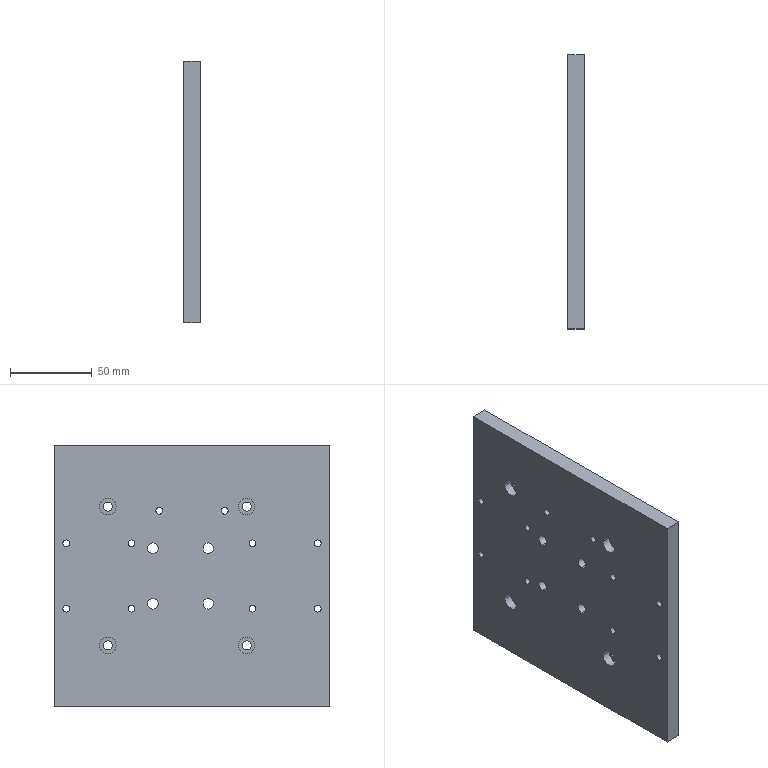Part | STEP file | 03-17 Suction mechanism fixing plate | 1 solid | 54 faces | box 10 x 168 x 160 mm | volume 264041 mm3 | cylinder 44 | plane 10 | commonest cylinder face diameters 4.2 x20 5.5 x8 6.5 x8 10 x8